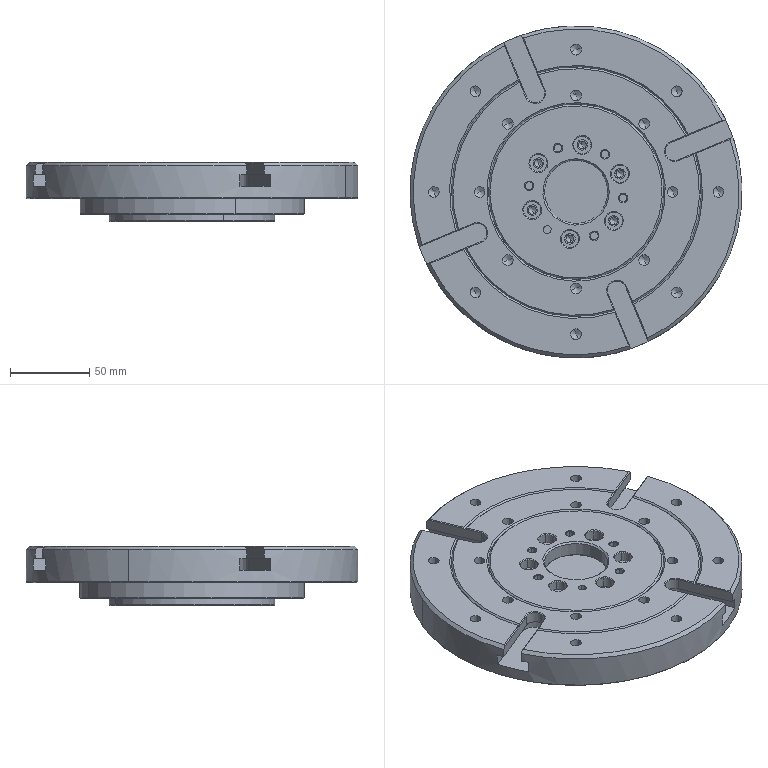NC program | Mastercam | posted with a generic post
Lines 3621 to 4738 of 4738:
(2.5 BM |TOOL - 15|DIA. OFF. - 15|LEN. - 15|TOOL DIA. - 2.5)
N7282 T15 M6
N7284 G0 G54 G90 X14.156 Y9.473 C49.947 B-90. S4500 M3
N7286 G43 H15 Z29.608
N7288 Y3.528
N7290 Z11.026
N7292 Z8.026
N7294 G1 Z6.026 F2000.
N7296 X14.166 Z5.862 F1000.
N7298 X14.193 Z5.699
N7300 X14.283 Z5.38
N7302 X14.292 Y3.524 Z5.322
N7304 X14.283 Y3.514 Z5.264
N7306 X14.22 Y3.48 Z5.155
N7308 X14.122 Y3.436 Z5.064
N7310 X14.012 Y3.391 Z5.007
N7312 X13.503 Y3.187 Z4.843 C50.063
N7314 X13.276 Y3.113 Z4.783 C50.113
N7316 X13.048 Y3.039 Z4.724 C50.163
N7318 X12.813 Y2.982 Z4.679 C50.213
N7320 X12.577 Y2.927 Z4.633 C50.234
N7322 X12.336 Y2.889 Z4.602 C50.255
N7324 X12.095 Y2.853 Z4.569 C50.247
N7326 X11.85 Y2.836 Z4.552 C50.24
N7328 X11.606 Y2.818 Z4.534 C50.232
N7330 X11.36 Z4.532 C50.224
N7332 X11.114 Y2.824 Z4.527 C50.161
N7334 X10.869 Y2.846 Z4.538 C50.098
N7336 X10.624 Y2.868 Z4.548 C50.035
N7338 X10.382 Y2.907 Z4.575 C49.971
N7340 X10.14 Y2.946 Z4.601 C49.908
N7342 X9.903 Y3. Z4.642 C49.845
N7344 X9.666 Y3.055 Z4.683 C49.782
N7346 X9.437 Y3.128 Z4.738 C49.719
N7348 X9.208 Y3.211 Z4.788 C49.558
N7350 X8.988 Y3.31 Z4.851 C49.398
N7352 X8.767 Y3.41 Z4.913 C49.237
N7354 X8.559 Y3.525 Z4.989 C49.077
N7356 X8.35 Y3.641 Z5.063 C48.916
N7358 X8.154 Y3.772 Z5.15 C48.755
N7360 X7.958 Y3.903 Z5.236 C48.595
N7362 X7.778 Y4.049 Z5.332 C48.434
N7364 X7.597 Y4.194 Z5.428 C48.274
N7366 X7.432 Y4.353 Z5.534 C48.113
N7368 X7.268 Y4.513 Z5.638 C47.953
N7370 X7.131 Y4.71 Z5.751 C47.785
N7372 X6.993 Y4.933 Z5.845 C47.412
N7374 X6.972 Y4.964 Z5.862 C47.357
N7376 X6.949 Y4.993 Z5.878 C47.301
N7378 X6.924 Y5.02 Z5.893 C47.246
N7380 X6.897 Y5.046 Z5.908 C47.191
N7382 X6.868 Y5.07 Z5.921 C47.136
N7384 X6.838 Y5.092 Z5.934 C47.081
N7386 X6.807 Y5.112 Z5.946 C47.026
N7388 X6.775 Y5.131 Z5.956 C46.971
N7390 X6.742 Y5.147 Z5.966 C46.917
N7392 X6.708 Y5.162 Z5.975 C46.863
N7394 X6.674 Y5.175 Z5.983 C46.81
N7396 X6.639 Y5.186 Z5.989 C46.756
N7398 X6.604 Y5.195 Z5.995 C46.703
N7400 X6.569 Y5.202 Z6. C46.651
N7402 X6.534 Y5.208 Z6.003 C46.599
N7404 X6.5 Y5.212 Z6.006 C46.547
N7406 X6.465 Y5.215 Z6.009 C46.496
N7408 X6.431 Y5.216 Z6.01 C46.445
N7410 X6.397 C46.394
N7412 X6.363 Y5.215 C46.344
N7414 X6.275 Y5.223 Z6.005 C46.216
N7416 X6.285 Y5.226 Z6.002 C46.202
N7418 X6.294 Y5.229 Z5.999 C46.189
N7420 X6.302 Y5.232 Z5.996 C46.176
N7422 X6.311 Y5.236 Z5.992 C46.162
N7424 X6.227 Y5.233 Z5.996 C46.035
N7426 X6.228 Y5.231 C46.03
N7428 X6.23 Y5.229 Z5.995 C46.026
N7430 X6.232 Y5.227 C46.022
N7432 X6.234 Y5.225 Z5.994 C46.017
N7434 X6.236 Y5.223 Z5.993 C46.013
N7436 X6.237 Y5.222 C46.009
N7438 X6.239 Y5.22 Z5.992 C46.004
N7440 X6.241 Y5.218 C46.
N7442 X6.243 Y5.216 Z5.991 C45.996
N7444 X6.244 Y5.214 Z5.99 C45.991
N7446 X6.246 Y5.212 C45.987
N7448 X6.248 Y5.21 Z5.989 C45.983
N7450 X6.25 Y5.209 C45.978
N7452 X6.251 Y5.207 Z5.988 C45.974
N7454 X6.253 Y5.205 C45.969
N7456 X6.255 Y5.203 Z5.987 C45.965
N7458 X6.257 Y5.201 Z5.986 C45.961
N7460 X6.259 Y5.199 C45.956
N7462 X6.26 Y5.197 Z5.985 C45.952
N7464 X6.262 Y5.196 C45.948
N7466 X6.264 Y5.194 Z5.984 C45.943
N7468 X6.266 Y5.192 Z5.983 C45.939
N7470 X6.267 Y5.19 C45.935
N7472 X6.269 Y5.188 Z5.982 C45.93
N7474 X6.271 Y5.186 C45.926
N7476 X6.273 Y5.184 Z5.981 C45.922
N7478 X6.274 Y5.183 C45.917
N7480 X6.276 Y5.181 Z5.98 C45.913
N7482 X6.278 Y5.179 Z5.979 C45.909
N7484 X6.28 Y5.177 C45.904
N7486 X6.281 Y5.175 Z5.978 C45.9
N7488 X6.283 Y5.169 Z5.976 C45.89
N7490 X6.284 Y5.164 Z5.974 C45.879
N7492 Y5.157 C45.867
N7494 Y5.151 C45.855
N7496 X6.287 Y5.15 Z5.97 C45.848
N7498 X6.29 Y5.149 Z5.966 C45.841
N7500 X6.293 Z5.961 C45.834
N7502 X6.296 Y5.148 Z5.957 C45.827
N7504 X6.299 Z5.953 C45.82
N7506 X6.307 Y5.152 Z5.957 C45.804
N7508 X6.276 Y5.097 Z5.989 C45.676
N7510 X6.278 Y5.096 Z5.986 C45.671
N7512 X6.281 Y5.095 Z5.984 C45.667
N7514 X6.283 Y5.094 Z5.982 C45.662
N7516 X6.285 Y5.093 Z5.98 C45.657
N7518 X6.287 Y5.092 Z5.978 C45.653
N7520 X6.289 Y5.09 Z5.976 C45.648
N7522 X6.297 Y5.077 Z5.972 C45.619
N7524 X6.305 Y5.063 Z5.969 C45.593
N7526 X6.298 Y4.73 Z6.205 C44.831
N7528 X6.303 Y4.403 Z6.404 C43.929
N7530 X6.309 Y4.055 Z6.603 C42.988
N7532 X6.321 Y3.757 Z6.758 C41.801
N7534 X6.341 Y3.441 Z6.91 C40.561
N7536 X6.373 Y3.158 Z7.033 C39.242
N7538 X6.415 Y2.862 Z7.153 C37.875
N7540 X6.47 Y2.596 Z7.255 C36.423
N7542 X6.555 Y2.322 Z7.333 C34.946
N7544 X6.652 Y2.101 Z7.396 C33.246
N7546 X6.768 Y1.878 Z7.455 C31.512
N7548 X6.913 Y1.686 Z7.493 C29.682
N7550 X7.079 Y1.501 Z7.527 C27.855
N7552 X7.266 Y1.325 Z7.557 C26.041
N7554 X7.325 Y1.282 Z7.562 C25.507
N7556 X7.344 Y1.273 Z7.563 C25.377
N7558 X7.363 Y1.265 Z7.562 C25.247
N7560 X7.383 Y1.258 Z7.558 C25.117
N7562 X7.403 Y1.251 Z7.551 C24.987
N7564 X7.424 Y1.247 Z7.541 C24.841
N7566 X7.444 Y1.244 Z7.529 C24.695
N7568 X7.465 Y1.242 Z7.515 C24.55
N7570 X7.485 Y1.241 Z7.499 C24.406
N7572 X7.505 Y1.24 Z7.482 C24.263
N7574 X7.525 Y1.241 Z7.462 C24.121
N7576 X7.545 Y1.243 Z7.442 C23.981
N7578 X7.564 Y1.246 Z7.42 C23.842
N7580 X7.582 Y1.251 Z7.398 C23.697
N7582 X7.601 Y1.257 Z7.374 C23.553
N7584 X7.618 Y1.264 Z7.35 C23.411
N7586 X7.635 Y1.272 Z7.326 C23.272
N7588 X7.81 Y1.274 Z7.077 C21.581
N7590 X7.975 Y1.291 Z6.846 C20.026
N7592 X8.12 Y1.293 Z6.662 C18.699
N7594 X8.28 Y1.286 Z6.465 C17.239
N7596 X8.447 Y1.251 Z6.276 C15.654
N7598 X8.6 Y1.196 Z6.092 C14.039
N7600 X8.672 Y1.149 Z6. C13.132
N7602 X8.745 Y1.106 Z5.912 C12.183
N7604 X8.852 Y1.012 Z5.763 C10.481
N7606 X8.937 Y.905 Z5.637 C8.736
N7608 X8.967 Y.836 Z5.584 C7.762
N7610 X8.997 Y.766 Z5.535 C6.787
N7612 X9.026 Y.634 Z5.465 C5.054
N7614 X9.025 Y.557 Z5.444 C4.088
N7616 X9.024 Y.481 Z5.427 C3.104
N7618 X8.993 Y.349 Z5.424 C1.364
N7620 X8.961 Y.276 Z5.435 C.415
N7622 X8.929 Y.202 Z5.45 C-.522
N7624 X8.843 Y.082 Z5.504 C-2.172
N7626 X8.737 Y-.024 Z5.576 C-3.805
N7628 X8.664 Y-.074 Z5.628 C-4.715
N7630 X8.59 Y-.122 Z5.684 C-5.626
N7632 X8.437 Y-.181 Z5.804 C-7.217
N7634 X8.188 Y-.254 Z6.015 C-9.499
N7636 X8.006 Y-.311 Z6.18 C-11.258
N7638 X7.923 Y-.333 Z6.264 C-12.084
N7640 X7.754 Y-.385 Z6.44 C-13.835
N7642 X7.669 Y-.419 Z6.536 C-14.696
N7644 X7.515 Y-.482 Z6.721 C-16.317
N7646 X7.373 Y-.543 Z6.912 C-17.934
N7648 X7.221 Y-.608 Z7.138 C-19.793
N7650 X7.157 Y-.599 Z7.2 C-20.143
N7652 X7.093 Y-.59 Z7.263 C-20.492
N7654 X7.028 Y-.579 Z7.326 C-20.841
N7656 X6.964 Y-.568 Z7.389 C-21.191
N7658 X6.899 Y-.556 Z7.452 C-21.54
N7660 X6.799 Y-.66 Z7.578 C-22.685
N7662 X6.793 Y-.674 Z7.593 C-22.82
N7664 X6.788 Y-.689 Z7.605 C-22.956
N7666 X6.783 Y-.704 Z7.614 C-23.091
N7668 X6.779 Y-.72 Z7.62 C-23.226
N7670 X6.775 Y-.737 Z7.624 C-23.361
N7672 X6.772 Y-.753 C-23.495
N7674 X6.77 Y-.769 Z7.622 C-23.629
N7676 X6.769 Y-.785 Z7.618 C-23.761
N7678 X6.768 Y-.8 Z7.612 C-23.893
N7680 Y-.815 Z7.604 C-24.023
N7682 X6.69 Y-.963 Z7.591 C-25.313
N7684 X6.621 Y-1.175 Z7.565 C-26.337
N7686 X6.564 Y-1.388 Z7.529 C-27.363
N7688 X6.516 Y-1.628 Z7.48 C-28.317
N7690 X6.47 Y-1.871 Z7.431 C-29.101
N7692 X6.437 Y-2.122 Z7.364 C-29.918
N7694 X6.403 Y-2.384 Z7.293 C-30.608
N7696 X6.376 Y-2.661 Z7.209 C-31.188
N7698 X6.352 Y-2.936 Z7.118 C-31.766
N7700 X6.341 Y-3.256 Z6.985 C-32.085
N7702 X6.327 Y-3.566 Z6.852 C-32.396
N7704 X6.32 Y-3.869 Z6.705 C-32.707
N7706 X6.31 Y-4.169 Z6.551 C-33.017
N7708 X6.304 Y-4.484 Z6.372 C-33.191
N7710 X6.295 Y-4.598 Z6.319 C-33.251
N7712 X6.293 Y-4.604 C-33.255
N7714 X6.291 Y-4.611 Z6.32 C-33.258
N7716 X6.289 Y-4.618 C-33.261
N7718 X6.287 Y-4.624 C-33.264
N7720 X6.285 Y-4.631 C-33.268
N7722 X6.283 Y-4.637 C-33.271
N7724 X6.281 Y-4.644 C-33.274
N7726 X6.279 Y-4.651 Z6.321 C-33.278
N7728 X6.277 Y-4.657 C-33.281
N7730 X6.275 Y-4.664 C-33.284
N7732 X6.273 Y-4.67 C-33.287
N7734 X6.271 Y-4.677 C-33.291
N7736 X6.269 Y-4.684 C-33.294
N7738 X6.267 Y-4.69 Z6.322 C-33.297
N7740 X6.266 Y-4.697 C-33.3
N7742 X6.264 Y-4.703 C-33.304
N7744 X6.262 Y-4.71 C-33.307
N7746 X6.26 Y-4.716 C-33.31
N7748 X6.258 Y-4.723 C-33.313
N7750 X6.256 Y-4.73 Z6.323 C-33.317
N7752 X6.254 Y-4.736 C-33.32
N7754 X6.252 Y-4.743 C-33.323
N7756 X6.312 Y-4.767 Z6.305 C-33.354
N7758 X6.319 Y-4.77 C-33.358
N7760 X6.325 Y-4.774 C-33.361
N7762 X7.175 Y-5.239 Z6.286 C-33.808
N7764 X7.319 Y-5.324 Z6.287
N7766 X7.474 Y-5.413 Z6.309
N7768 X7.63 Y-5.5 Z6.352
N7770 X7.782 Y-5.58 Z6.416
N7772 X7.922 Y-5.65 Z6.5
N7774 X8.042 Y-5.706 Z6.605
N7776 X8.135 Y-5.742 Z6.73
N7778 X8.194 Y-5.756 Z6.875
N7780 X8.291 Z7.279
N7782 X8.37 Z7.687
N7784 X8.423 Z8.098
N7786 X8.443 Z8.511
N7788 G0 Z10.511
N7790 Z13.511
N7792 Z28.6
N7794 Y-12.184
N7796 Z30.435
N7798 X7.794 Y6.335
N7800 C-78.812
N7802 Y3.076
N7804 Z14.777
N7806 Z11.777
N7808 G1 Z9.777 F2000.
N7810 X7.766 Z9.367 F1000.
N7812 X7.691 Z8.962
N7814 X7.579 Z8.563
N7816 X7.444 Z8.173
N7818 X7.384 Y3.051 Z8.043
N7820 X7.311 Y2.984 Z7.932
N7822 X7.229 Y2.883 Z7.841
N7824 X7.143 Y2.755 Z7.77
N7826 X7.057 Y2.611 Z7.719
N7828 X6.974 Y2.458 Z7.689
N7830 X6.898 Y2.304 Z7.679
N7832 X6.834 Y2.16 Z7.69
N7834 X6.789 Y2.083 Z7.698 C-79.057
N7836 X6.744 Y2.01 Z7.705 C-79.331
N7838 X6.699 Y1.938 Z7.714 C-79.606
N7840 X6.654 Y1.866 Z7.724 C-79.88
N7842 X6.609 Y1.798 Z7.734 C-80.18
N7844 X6.563 Y1.73 Z7.744 C-80.481
N7846 X6.518 Y1.669 Z7.755 C-80.817
N7848 X6.473 Y1.607 Z7.766 C-81.154
N7850 X6.442 Y1.565 Z7.775 C-81.384
N7852 X6.412 Y1.523 Z7.784 C-81.613
N7854 X6.381 Y1.452 Z7.791 C-81.979
N7856 X6.343 Y1.395 Z7.802 C-82.297
N7858 X6.305 Y1.337 Z7.813 C-82.614
N7860 X6.276 Y1.266 Z7.82 C-83.021
N7862 X6.243 Y1.209 Z7.829 C-83.356
N7864 X6.21 Y1.157 Z7.839 C-83.721
N7866 X6.187 Y1.09 Z7.843 C-84.157
N7868 X6.16 Y1.038 Z7.851 C-84.513
N7870 X6.133 Y.972 Z7.859 C-84.951
N7872 X6.111 Y.917 Z7.864 C-85.301
N7874 X6.089 Y.863 Z7.871 C-85.652
N7876 X6.067 Y.809 Z7.878 C-86.003
N7878 X6.052 Y.743 Z7.881 C-86.446
N7880 X6.035 Y.69 Z7.886 C-86.801
N7882 X6.018 Y.641 Z7.892 C-87.178
N7884 X6.004 Y.578 Z7.895 C-87.651
N7886 X5.992 Y.528 Z7.898 C-88.029
N7888 X5.981 Y.465 Z7.902 C-88.504
N7890 X5.974 Y.413 Z7.904 C-88.867
N7892 X5.967 Y.361 Z7.906 C-89.23
N7894 X5.959 Y.309 Z7.91 C-89.593
N7896 X5.955 Y.244 Z7.911 C-90.055
N7898 X5.952 Y.192 Z7.913 C-90.421
N7900 X5.95 Y.141 Z7.915 C-90.788
N7902 X5.954 Y.076 Z7.914 C-91.255
N7904 X5.957 Y.024 C-91.624
N7906 X5.96 Y-.04 Z7.915 C-92.09
N7908 X5.967 Y-.088 Z7.913 C-92.479
N7910 X5.974 Y-.136 Z7.912 C-92.868
N7912 X5.981 Y-.183 C-93.257
N7914 X5.994 Y-.244 Z7.909 C-93.742
N7916 X6.006 Y-.293 Z7.907 C-94.129
N7918 X6.018 Y-.341 C-94.516
N7920 X6.035 Y-.401 Z7.903 C-95.003
N7922 X6.052 Y-.449 Z7.9 C-95.393
N7924 X6.069 Y-.497 Z7.898 C-95.783
N7926 X6.091 Y-.558 Z7.894 C-96.265
N7928 X6.113 Y-.606 Z7.889 C-96.654
N7930 X6.135 Y-.655 Z7.886 C-97.043
N7932 X6.16 Y-.715 Z7.882 C-97.52
N7934 X6.187 Y-.765 Z7.876 C-97.89
N7936 X6.214 Y-.815 Z7.872 C-98.26
N7938 X6.244 Y-.878 Z7.867 C-98.722
N7940 X6.277 Y-.928 Z7.86 C-99.105
N7942 X6.31 Y-.978 Z7.855 C-99.487
N7944 X6.343 Y-1.039 Z7.849 C-99.948
N7946 X6.381 Y-1.09 Z7.841 C-100.313
N7948 X6.419 Y-1.14 Z7.835 C-100.678
N7950 X6.447 Y-1.208 Z7.833 C-101.116
N7952 X6.486 Y-1.25 Z7.825 C-101.432
N7954 X6.525 Y-1.293 Z7.817 C-101.748
N7956 X6.563 Y-1.335 Z7.81 C-102.064
N7958 X6.603 Y-1.388 Z7.803 C-102.436
N7960 X6.646 Y-1.43 Z7.795 C-102.748
N7962 X6.689 Y-1.471 Z7.787 C-103.06
N7964 X6.726 Y-1.525 Z7.781 C-103.391
N7966 X6.77 Y-1.564 Z7.772 C-103.668
N7968 X6.814 Y-1.605 Z7.763 C-103.929
N7970 X6.859 Y-1.647 Z7.754 C-104.191
N7972 X6.899 Y-1.703 Z7.748 C-104.518
N7974 X6.949 Y-1.741 Z7.738 C-104.794
N7976 X6.999 Y-1.78 Z7.729 C-105.07
N7978 X7.036 Y-1.838 Z7.726 C-105.398
N7980 X7.091 Y-1.878 Z7.714 C-105.654
N7982 X7.147 Y-1.919 Z7.703 C-105.91
N7984 X7.203 Y-1.96 Z7.692 C-106.164
N7986 X7.258 Y-2. Z7.681 C-106.418
N7988 X7.309 Y-2.055 Z7.673 C-106.706
N7990 X7.369 Y-2.092 Z7.662 C-106.961
N7992 X7.429 Y-2.13 Z7.65 C-107.21
N7994 X7.479 Y-2.185 Z7.644 C-107.484
N7996 X7.542 Y-2.219 Z7.632 C-107.73
N7998 X7.606 Y-2.254 Z7.62 C-107.976
N8000 X7.657 Y-2.308 Z7.612 C-108.216
N8002 X7.724 Y-2.344 Z7.6 C-108.441
N8004 X7.79 Y-2.38 Z7.587 C-108.666
N8006 X7.857 Y-2.415 Z7.575 C-108.892
N8008 X7.917 Y-2.461 Z7.566 C-109.125
N8010 X7.986 Y-2.493 Z7.554 C-109.35
N8012 X8.043 Y-2.541 Z7.546 C-109.582
N8014 X8.112 Y-2.569 Z7.534 C-109.793
N8016 X8.18 Y-2.597 Z7.523 C-110.005
N8018 X8.249 Y-2.628 Z7.512 C-110.202
N8020 X8.299 Y-2.679 Z7.506 C-110.409
N8022 X8.38 Y-2.71 Z7.493 C-110.633
N8024 X8.461 Y-2.741 Z7.48 C-110.857
N8026 X8.542 Y-2.774 Z7.467 C-111.066
N8028 X8.616 Y-2.815 Z7.456 C-111.271
N8030 X8.7 Y-2.845 Z7.443 C-111.479
N8032 X8.784 Y-2.876 Z7.43 C-111.683
N8034 X8.845 Y-2.908 Z7.422 C-111.844
N8036 X8.915 Y-2.931 Z7.412 C-112.009
N8038 X8.986 Y-2.954 Z7.402 C-112.173
N8040 X9.057 Y-2.998 Z7.394 C-112.37
N8042 X9.147 Y-3.023 Z7.382 C-112.573
N8044 X9.237 Y-3.048 Z7.37 C-112.776
N8046 X9.311 Y-3.085 Z7.362 C-112.963
N8048 X9.404 Y-3.105 Z7.351 C-113.165
N8050 X9.496 Y-3.13 Z7.339 C-113.33
N8052 X9.589 Y-3.156 Z7.327 C-113.495
N8054 X9.666 Y-3.197 Z7.317 C-113.653
N8056 X9.76 Y-3.226 Z7.306 C-113.822
N8058 X9.865 Y-3.252 Z7.293 C-113.979
N8060 X9.969 Y-3.277 Z7.28 C-114.136
N8062 X10.055 Y-3.316 Z7.27 C-114.279
N8064 X10.167 Y-3.338 Z7.258 C-114.443
N8066 X10.278 Y-3.36 Z7.246 C-114.607
N8068 X10.37 Y-3.394 Z7.237 C-114.752
N8070 X10.465 Y-3.409 Z7.228 C-114.89
N8072 X10.559 Y-3.424 Z7.219 C-115.027
N8074 X10.654 Y-3.439 Z7.211 C-115.164
N8076 X10.728 Y-3.466 Z7.205 C-115.28
N8078 X10.825 Y-3.477 Z7.198 C-115.418
N8080 X10.921 Y-3.489 Z7.191 C-115.556
N8082 X11.018 Y-3.5 Z7.184 C-115.694
N8084 X11.098 Y-3.526 Z7.179 C-115.817
N8086 X11.211 Y-3.536 Z7.173 C-115.976
N8088 X11.313 Y-3.547 Z7.168 C-116.12
N8090 X11.426 Y-3.556 Z7.161 C-116.263
N8092 X11.522 Y-3.574 Z7.156 C-116.388
N8094 X11.63 Y-3.585 Z7.15 C-116.492
N8096 X11.739 Y-3.595 Z7.144 C-116.597
N8098 X11.828 Y-3.614 Z7.138 C-116.667
N8100 X11.926 Y-3.623 Z7.132 C-116.742
N8102 X12.025 Y-3.632 Z7.127 C-116.812
N8104 X12.123 Y-3.642 Z7.121 C-116.882
N8106 X12.199 Y-3.657 Z7.117 C-116.937
N8108 X12.298 Y-3.663 Z7.113 C-117.007
N8110 X12.397 Y-3.669 Z7.11 C-117.077
N8112 X12.496 Y-3.674 Z7.106 C-117.147
N8114 X12.595 Y-3.68 Z7.102 C-117.216
N8116 X12.672 Y-3.688 Z7.101 C-117.271
N8118 X12.771 Y-3.69 Z7.099 C-117.34
N8120 X12.87 Y-3.692 Z7.097 C-117.41
N8122 X12.947 Y-3.703 Z7.096 C-117.464
N8124 X13.047 Y-3.702 C-117.534
N8126 X13.146 Y-3.701 Z7.095 C-117.603
N8128 X13.246 Y-3.699 C-117.673
N8130 X13.323 Y-3.708 C-117.728
N8132 X13.423 Y-3.703 Z7.097 C-117.797
N8134 X13.522 Y-3.698 Z7.099 C-117.866
N8136 X13.622 Y-3.694 Z7.1 C-117.935
N8138 X13.699 Y-3.695 Z7.102 C-117.989
N8140 X13.799 Y-3.687 Z7.105 C-118.059
N8142 X13.9 Y-3.678 Z7.109 C-118.128
N8144 X14. Y-3.67 Z7.112 C-118.198
N8146 X14.1 Y-3.661 Z7.116 C-118.267
N8148 X14.213 Y-3.652 Z7.121 C-118.346
N8150 X14.338 Y-3.641 Z7.126 C-118.421
N8152 X14.462 Y-3.63 Z7.13 C-118.497
N8154 X14.586 Y-3.623 Z7.133 C-118.54
N8156 X14.711 Y-3.617 Z7.136 C-118.583
N8158 X14.835 Y-3.615 Z7.137 C-118.594
N8160 X14.959 Y-3.614 C-118.604
N8162 X15.084
N8164 X15.208
N8166 X15.332
N8168 X15.457
N8170 X15.581
N8172 X15.705
N8174 X15.83
N8176 X15.954
N8178 X16.078
N8180 X16.203
N8182 X16.327
N8184 X16.451
N8186 X15.879 Y-3.699 Z7.207 C-118.726
N8188 X16.004 Y-3.694 Z7.209 C-118.768
N8190 X16.129 Y-3.688 Z7.211 C-118.811
N8192 X16.254 Y-3.683 Z7.214 C-118.853
N8194 X16.379 Y-3.672 Z7.218 C-118.932
N8196 X16.504 Y-3.661 Z7.223 C-119.012
N8198 X16.629 Y-3.65 Z7.227 C-119.091
N8200 X16.754 Y-3.633 Z7.234 C-119.208
N8202 X16.879 Y-3.616 Z7.241 C-119.325
N8204 X17.004 Y-3.6 Z7.248 C-119.442
N8206 X17.109 Y-3.583 Z7.255 C-119.573
N8208 X17.253 Y-3.56 Z7.263 C-119.754
N8210 X17.367 Y-3.549 Z7.267 C-119.897
N8212 X17.521 Y-3.523 Z7.275 C-120.155
N8214 X17.635 Y-3.512 Z7.278 C-120.348
N8216 X17.789 Y-3.495 Z7.282 C-120.609
N8218 X17.902 Y-3.476 Z7.288 C-120.904
N8220 X18.055 Y-3.447 Z7.295 C-121.304
N8222 X18.166 Y-3.434 Z7.298 C-121.6
N8224 X18.318 Y-3.403 Z7.306 C-122.08
N8226 X18.427 Y-3.389 Z7.309 C-122.434
N8228 X18.536 Y-3.374 Z7.312 C-122.787
N8230 X18.684 Y-3.348 Z7.317 C-123.358
N8232 X18.831 Y-3.325 Z7.322 C-123.932
N8234 X18.935 Y-3.313 C-124.349
N8236 X19.039 Y-3.292 Z7.327 C-124.827
N8238 X19.174 Y-3.262 Z7.329 C-125.448
N8240 X19.305 Y-3.247 Z7.332 C-126.083
N8242 X19.376 Y-3.23 Z7.335 C-126.489
N8244 X19.447 Y-3.214 Z7.338 C-126.896
N8246 X19.56 Y-3.187 Z7.341 C-127.541
N8248 X19.655 Y-3.169 Z7.343 C-128.108
N8250 X19.79 Y-3.136 Z7.347 C-128.963
N8252 X19.881 Y-3.118 Z7.349 C-129.563
N8254 X19.972 Y-3.1 Z7.35 C-130.163
N8256 X20.088 Y-3.072 Z7.352 C-130.997
N8258 X20.166 Y-3.055 Z7.354 C-131.572
N8260 X20.263 Y-3.038 C-132.323
N8262 X20.324 Y-3.025 Z7.355 C-132.804
N8264 X20.384 Y-3.013 Z7.356 C-133.285
N8266 X20.502 Y-2.99 Z7.354 C-134.253
N8268 X20.579 Y-2.974 Z7.355 C-134.929
N8270 X20.675 Y-2.956 Z7.353 C-135.804
N8272 X20.731 Y-2.946 Z7.352 C-136.33
N8274 X20.786 Y-2.938 C-136.856
N8276 X20.885 Y-2.92 Z7.349 C-137.842
N8278 X20.947 Y-2.911 Z7.348 C-138.474
N8280 X21.036 Y-2.898 Z7.343 C-139.428
N8282 X21.093 Y-2.891 Z7.341 C-140.058
N8284 X21.167 Y-2.883 Z7.334 C-140.903
N8286 X21.207 Y-2.879 Z7.332 C-141.39
N8288 X21.246 Y-2.876 Z7.33 C-141.878
N8290 X21.268 Y-2.873 Z7.326 C-142.152
N8292 X21.296 Y-2.253 Z7.512 C-146.739
N8294 X21.324 Y-1.621 Z7.645 C-151.327
N8296 X21.351 Y-.983 Z7.726 C-155.914
N8298 X21.379 Y-.342 Z7.753 C-160.502
N8300 X21.388 Y-.344 Z7.749 C-160.797
N8302 X21.392 Y-.351 Z7.745 C-161.525
N8304 X21.395 Y-.36 Z7.742 C-162.241
N8306 X21.399 Y-.369 C-162.957
N8308 X21.403 Y-.38 C-163.661
N8310 X21.406 Y-.391 Z7.745 C-164.365
N8312 X21.411 Y-.419 Z7.741 C-165.36
N8314 X21.415 Y-.436 Z7.738 C-166.015
N8316 X21.419 Y-.453 Z7.737 C-166.67
N8318 X21.423 Y-.47 C-167.331
N8320 X21.428 Y-.495 Z7.74 C-168.344
N8322 X21.433 Y-.511 Z7.735 C-169.01
N8324 X21.437 Y-.527 Z7.732 C-169.675
N8326 X21.441 Y-.542 Z7.731 C-170.341
N8328 X21.446 Y-.561 C-170.989
N8330 X21.45 Y-.579 Z7.732 C-171.637
N8332 X21.456 Y-.608 Z7.728 C-172.631
N8334 X21.461 Y-.63 Z7.724 C-173.256
N8336 X21.466 Y-.652 Z7.722 C-173.881
N8338 X21.471 Y-.674 C-174.506
N8340 X21.476 Y-.704 Z7.723 C-175.35
N8342 X21.481 Y-.724 Z7.721 C-175.928
N8344 X21.485 Y-.749 Z7.719 C-176.481
N8346 X21.49 Y-.773 C-177.034
N8348 X21.495 Y-.798 Z7.72 C-177.586
N8350 X21.499 Y-.822 Z7.722 C-178.139
N8352 X21.504 Y-.847 Z7.726 C-178.692
N8354 X21.509 Y-.885 Z7.734 C-179.534
N8356 X21.514 Y-.909 Z7.733 C-180.087
N8358 X21.519 Y-.936 Z7.734 C-180.622
N8360 X21.524 Y-.963 Z7.736 C-181.158
N8362 X21.529 Y-.99 Z7.739 C-181.693
N8364 X21.534 Y-1.017 Z7.743 C-182.228
N8366 X21.539 Y-1.045 Z7.749 C-182.764
N8368 X21.546 Y-1.086 Z7.759 C-183.579
N8370 X21.551 Y-1.113 Z7.761 C-184.115
N8372 X21.556 Y-1.142 Z7.763 C-184.633
N8374 X21.561 Y-1.172 Z7.767 C-185.152
N8376 X21.567 Y-1.204 Z7.772 C-185.654
N8378 X21.572 Y-1.236 Z7.777 C-186.156
N8380 X21.577 Y-1.268 Z7.785 C-186.658
N8382 X21.583 Y-1.317 Z7.798 C-187.423
N8384 X21.588 Y-1.349 Z7.801 C-187.924
N8386 X21.594 Y-1.38 Z7.805 C-188.426
N8388 X21.599 Y-1.412 Z7.81 C-188.928
N8390 X21.604 Y-1.444 Z7.817 C-189.429
N8392 X21.61 Y-1.476 Z7.825 C-189.931
N8394 X21.615 Y-1.507 Z7.834 C-190.433
N8396 X21.621 Y-1.539 Z7.844 C-190.934
N8398 X21.629 Y-1.587 Z7.853 C-191.699
N8400 X21.634 Y-1.618 Z7.859 C-192.201
N8402 X21.64 Y-1.65 Z7.867 C-192.702
N8404 X21.646 Y-1.681 Z7.875 C-193.204
N8406 X21.651 Y-1.712 Z7.885 C-193.705
N8408 X21.657 Y-1.743 Z7.896 C-194.207
N8410 X21.663 Y-1.774 Z7.908 C-194.708
N8412 X21.671 Y-1.821 Z7.921 C-195.473
N8414 X21.677 Y-1.852 Z7.929 C-195.975
N8416 X21.683 Y-1.883 Z7.938 C-196.476
N8418 X21.688 Y-1.913 Z7.948 C-196.978
N8420 X21.694 Y-1.944 Z7.96 C-197.48
N8422 X21.7 Y-1.974 Z7.973 C-197.983
N8424 X21.706 Y-2.005 Z7.987 C-198.485
N8426 X21.712 Y-2.051 Z8.004 C-199.251
N8428 X21.718 Y-2.08 Z8.014 C-199.754
N8430 X21.724 Y-2.11 Z8.025 C-200.256
N8432 X21.73 Y-2.14 Z8.038 C-200.758
N8434 X21.736 Y-2.17 Z8.051 C-201.261
N8436 X21.742 Y-2.199 Z8.066 C-201.763
N8438 X21.748 Y-2.228 Z8.082 C-202.267
N8440 X21.756 Y-2.273 Z8.1 C-203.036
N8442 X21.763 Y-2.301 Z8.112 C-203.54
N8444 X21.769 Y-2.33 Z8.125 C-204.043
N8446 X21.775 Y-2.359 Z8.139 C-204.547
N8448 X21.781 Y-2.387 Z8.154 C-205.051
N8450 X21.787 Y-2.416 Z8.171 C-205.555
N8452 X21.793 Y-2.444 Z8.189 C-206.058
N8454 X21.801 Y-2.487 Z8.21 C-206.828
N8456 X21.808 Y-2.514 Z8.224 C-207.333
N8458 X21.814 Y-2.542 Z8.238 C-207.838
N8460 X21.82 Y-2.569 Z8.254 C-208.343
N8462 X21.826 Y-2.596 Z8.272 C-208.848
N8464 X21.833 Y-2.624 Z8.29 C-209.354
N8466 X21.839 Y-2.651 Z8.31 C-209.859
N8468 X21.846 Y-2.692 Z8.335 C-210.631
N8470 X21.852 Y-2.718 Z8.35 C-211.136
N8472 X21.858 Y-2.744 Z8.367 C-211.641
N8474 X21.865 Y-2.77 Z8.385 C-212.152
N8476 X21.871 Y-2.795 Z8.404 C-212.662
N8478 X21.877 Y-2.82 Z8.424 C-213.173
N8480 X21.884 Y-2.845 Z8.446 C-213.684
N8482 X21.892 Y-2.882 Z8.472 C-214.465
N8484 X21.899 Y-2.907 Z8.49 C-214.975
N8486 X21.905 Y-2.931 Z8.508 C-215.486
N8488 X21.912 Y-2.955 Z8.527 C-215.997
N8490 X21.918 Y-2.979 Z8.548 C-216.507
N8492 X21.924 Y-3. Z8.571 C-217.033
N8494 X21.931 Y-3.021 Z8.595 C-217.56
N8496 X21.939 Y-3.052 Z8.626 C-218.365
N8498 X21.946 Y-3.072 Z8.645 C-218.891
N8500 X21.952 Y-3.092 Z8.666 C-219.417
N8502 X21.959 Y-3.112 Z8.688 C-219.944
N8504 X21.965 Y-3.132 Z8.711 C-220.47
N8506 X21.971 Y-3.155 Z8.734 C-220.979
N8508 X21.978 Y-3.177 Z8.759 C-221.488
N8510 X21.987 Y-3.211 Z8.79 C-222.267
N8512 X21.993 Y-3.236 Z8.809 C-222.753
N8514 X21.999 Y-3.262 Z8.829 C-223.239
N8516 X22.006 Y-3.287 Z8.85 C-223.726
N8518 X22.012 Y-3.313 Z8.873 C-224.212
N8520 X22.019 Y-3.338 Z8.896 C-224.698
N8522 X22.025 Y-3.363 Z8.921 C-225.184
N8524 X22.034 Y-3.401 Z8.952 C-225.929
N8526 X22.041 Y-3.431 Z8.97 C-226.383
N8528 X22.047 Y-3.461 Z8.989 C-226.837
N8530 X22.053 Y-3.496 Z9.008 C-227.259
N8532 X22.06 Y-3.532 Z9.027 C-227.68
N8534 X22.066 Y-3.567 Z9.048 C-228.102
N8536 X22.072 Y-3.603 Z9.069 C-228.523
N8538 X22.066 Y-3.633 Z9.096 C-228.887
N8540 X22.06 Y-3.663 Z9.124 C-229.25
N8542 X22.052 Y-3.702 Z9.161 C-229.723
N8544 X22.044 Y-3.74 Z9.2 C-230.196
N8546 X22.036 Y-3.778 Z9.24 C-230.668
N8548 X22.028 Y-3.816 Z9.281 C-231.141
N8550 X22.02 Y-3.853 Z9.324 C-231.614
N8552 X22.012 Y-3.89 Z9.368 C-232.086
N8554 X22.004 Y-3.926 Z9.413 C-232.559
N8556 X21.996 Y-3.962 Z9.46 C-233.032
N8558 X21.993 Y-4.121 Z9.489
N8560 X22.006 Y-4.287 Z9.535
N8562 X22.034 Y-4.453 Z9.597
N8564 X22.076 Y-4.608 Z9.672
N8566 X22.133 Y-4.745 Z9.758
N8568 X22.205 Y-4.854 Z9.854
N8570 X22.291 Y-4.926 Z9.957
N8572 X22.391 Y-4.952 Z10.065
N8574 X22.651 Z10.365
N8576 X22.769 Z10.53
N8578 X22.873 Z10.703
N8580 X22.961 Z10.883
N8582 X23.028 Z11.068
N8584 X23.071 Z11.257
N8586 X23.087 Z11.45
N8588 G0 Z13.45
N8590 Z16.45
N8592 Z29.768
N8594 Y-8.96
N8596 Z31.036
N8598 X-17.141 Y-8.869
N8600 C-180. B-270.
N8602 Z6.928
N8604 Z3.928
N8606 G1 Z1.928 F2000.
N8608 X-17.127 Y-8.867 Z1.734 F1000.
N8610 X-17.086 Y-8.862 Z1.542
N8612 X-17.023 Y-8.854 Z1.355
N8614 X-16.939 Y-8.844 Z1.172
N8616 X-16.84 Y-8.831 Z.996
N8618 X-16.728 Y-8.817 Z.827
N8620 X-16.479 Y-8.785 Z.517
N8622 X-16.383 Y-8.747 Z.413
N8624 X-16.295 Y-8.664 Z.327
N8626 X-16.215 Y-8.544 Z.259
N8628 X-16.147 Y-8.399 Z.206
N8630 X-16.089 Y-8.236 Z.171
N8632 X-16.046 Y-8.066 Z.152
N8634 X-16.016 Y-7.897 Z.149
N8636 X-16.003 Y-7.74 Z.163
N8638 X-15.985 Y-7.246 Z.234
N8640 X-15.968 Y-6.751 Z.305
N8642 X-15.95 Y-6.258 Z.376
N8644 X-15.933 Y-5.765 Z.447
N8646 X-15.916 Y-5.273 Z.518
N8648 X-15.898 Y-4.78 Z.589
N8650 X-15.897 Y-4.742 Z.594
N8652 X-15.896 Y-4.704 Z.597
N8654 X-15.895 Y-4.665 Z.598
N8656 X-15.894 Y-4.627 Z.597
N8658 X-15.893 Y-4.589 Z.594
N8660 Y-4.551 Z.59
N8662 Y-4.513 Z.583
N8664 X-15.894 Y-4.476 Z.575
N8666 Y-4.438 Z.565
N8668 X-15.895 Y-4.402 Z.554
N8670 X-15.896 Y-4.366 Z.541
N8672 X-15.897 Y-4.33 Z.526
N8674 X-15.899 Y-4.296 Z.509
N8676 X-15.905 Y-4.19 Z.453
N8678 X-15.91 Y-4.075 Z.401
N8680 X-15.915 Y-3.955 Z.356
N8682 X-15.916 Y-3.911 Z.342
N8684 X-15.918 Y-3.867 Z.327
N8686 X-15.919 Y-3.741 Z.297
N8688 X-15.92 Y-3.612 Z.274
N8690 Y-3.565 Z.268
N8692 Y-3.518 Z.262
N8694 X-15.918 Y-3.388 Z.255
N8696 X-15.916 Y-3.257 Z.256
N8698 X-15.914 Y-3.21 Z.259
N8700 X-15.912 Y-3.163 Z.263
N8702 X-15.907 Y-3.035 Z.28
N8704 X-15.901 Y-2.91 Z.304
N8706 X-15.898 Y-2.873 Z.314
N8708 X-15.895 Y-2.836 Z.323
N8710 X-15.887 Y-2.683 Z.372
N8712 X-15.884 Y-2.64 Z.386
N8714 X-15.881 Y-2.605 Z.388
N8716 Y-2.572 Z.393
N8718 Y-2.537 Z.398
N8720 X-15.88 Y-2.502 Z.402
N8722 X-15.879 Y-2.465 Z.405
N8724 X-15.877 Y-2.428 Z.408
N8726 X-15.874 Y-2.389 Z.41
N8728 X-15.871 Y-2.349 Z.411
N8730 X-15.867 Y-2.307
N8732 X-15.821 Y-2.228 Z.442
N8734 X-15.785 Y-2.19 Z.468
N8736 X-15.74 Y-2.113 Z.503
N8738 X-15.704 Y-2.073 Z.533
N8740 X-15.669 Y-2.034 Z.562
N8742 X-15.625 Y-1.96 Z.604
N8744 X-15.59 Y-1.924 Z.638
N8746 X-15.557 Y-1.889 Z.671
N8748 X-15.515 Y-1.819 Z.719
N8750 X-15.483 Y-1.787 Z.755
N8752 X-15.452 Y-1.756 Z.79
N8754 X-15.424 Y-1.737 Z.819
N8756 X-15.386 Y-1.675 Z.877
N8758 X-15.337 Y-1.596 Z.951
N8760 X-15.327 Y-1.558 Z.98
N8762 X-15.317 Y-1.517 Z1.004
N8764 X-15.307 Y-1.474 Z1.025
N8766 X-15.295 Y-1.43 Z1.042
N8768 X-15.284 Y-1.385 Z1.056
N8770 X-15.272 Y-1.339 Z1.065
N8772 X-15.26 Y-1.292 Z1.071
N8774 X-15.249 Y-1.246 Z1.073
N8776 X-15.238 Y-1.2
N8778 X-15.227 Y-1.154 Z1.069
N8780 X-15.217 Y-1.109 Z1.063
N8782 X-15.088 Y-.879 Z1.096
N8784 X-14.959 Y-.648 Z1.13
N8786 X-14.911 Y-.545 Z1.145
N8788 X-14.904 Y-.514 Z1.149
N8790 X-14.897 Y-.484 Z1.153
N8792 X-14.893 Y-.454 Z1.158
N8794 X-14.89 Y-.423 Z1.162
N8796 Y-.392 Z1.167
N8798 Y-.361 Z1.171
N8800 X-14.894 Y-.331 Z1.175
N8802 X-14.897 Y-.3 Z1.18
N8804 X-14.905 Y-.27 Z1.184
N8806 X-14.912 Y-.24 Z1.188
N8808 X-14.922 Y-.212 Z1.193
N8810 X-14.933 Y-.183 Z1.197
N8812 X-14.946 Y-.155 Z1.201
N8814 X-14.96 Y-.128 Z1.205
N8816 X-14.977 Y-.102 Z1.208
N8818 X-14.993 Y-.076 Z1.212
N8820 X-15.013 Y-.053 Z1.216
N8822 X-15.032 Y-.029 Z1.219
N8824 X-15.054 Y-.007 Z1.222
N8826 X-15.077 Y.014 Z1.225
N8828 X-15.101 Y.033 Z1.228
N8830 X-15.125 Y.051 Z1.231
N8832 X-15.152 Y.067 Z1.233
N8834 X-15.178 Y.083 Z1.235
N8836 X-15.206 Y.096 Z1.237
N8838 X-15.234 Y.109 Z1.239
N8840 X-15.263 Y.118 Z1.24
N8842 X-15.293 Y.128 Z1.242
N8844 Y.14 Z1.248
N8846 X-15.298 Y.139
N8848 X-15.303
N8850 X-15.309
N8852 X-15.314
N8854 X-15.319
N8856 X-15.324
N8858 X-15.329
N8860 X-15.335
N8862 X-15.34
N8864 X-15.345
N8866 X-15.35
N8868 X-15.355
N8870 X-15.361
N8872 X-15.366
N8874 X-15.371
N8876 X-15.376
N8878 X-15.382 Z1.247
N8880 X-15.387
N8882 X-15.392
N8884 X-15.397
N8886 X-15.402
N8888 X-15.408
N8890 X-15.413
N8892 X-15.418
N8894 X-15.423
N8896 X-15.428
N8898 X-15.434
N8900 X-15.439
N8902 X-15.444
N8904 X-15.449
N8906 X-15.454
N8908 X-15.46
N8910 X-15.465
N8912 X-15.47
N8914 X-15.475
N8916 X-15.48 Z1.246
N8918 X-15.486
N8920 X-15.491
N8922 X-15.496
N8924 X-15.501
N8926 X-15.506
N8928 X-15.512
N8930 X-15.517
N8932 X-15.522
N8934 X-15.527 Y.138
N8936 X-15.533
N8938 X-15.538
N8940 X-15.543
N8942 X-15.548
N8944 X-15.553
N8946 X-15.559
N8948 X-15.564
N8950 X-15.569
N8952 X-15.573 Y.128 Z1.242
N8954 X-15.598 Y.12 Z1.24
N8956 X-15.624 Y.111 Z1.239
N8958 X-15.649 Y.101 Z1.238
N8960 X-15.674 Y.09 Z1.236
N8962 X-15.698 Y.077 Z1.234
N8964 X-15.721 Y.064 Z1.232
N8966 X-15.744 Y.049 Z1.23
N8968 X-15.766 Y.034 Z1.228
N8970 X-15.787 Y.017 Z1.226
N8972 X-15.808 Y0. Z1.223
N8974 X-15.828 Y-.019 Z1.22
N8976 X-15.847 Y-.038 Z1.218
N8978 X-15.934 Y-.172 Z1.198
N8980 X-16.119 Y-.506 Z1.15
N8982 X-16.332 Y-.886 Z1.095
N8984 X-16.545 Y-1.265 Z1.041
N8986 X-16.758 Y-1.644 Z.986
N8988 X-16.78 Y-1.68
N8990 X-16.804 Y-1.714 Z.987
N8992 X-16.83 Y-1.746 Z.988
N8994 X-16.859 Y-1.776 Z.989
N8996 X-16.89 Y-1.804 Z.991
N8998 X-16.922 Y-1.829 Z.993
N9000 X-16.956 Y-1.852 Z.995
N9002 X-16.992 Y-1.873 Z.997
N9004 X-17.028 Y-1.891 Z1.
N9006 X-17.065 Y-1.907 Z1.003
N9008 X-17.246 Y-2.024 Z.986
N9010 X-17.426 Y-2.145 Z.974
N9012 X-17.447 Y-2.19 Z.954
N9014 X-17.463 Y-2.235 Z.922
N9016 X-17.477 Y-2.276 Z.879
N9018 X-17.487 Y-2.314 Z.827
N9020 X-17.492 Y-2.348 Z.771
N9022 X-17.494 Y-2.38 Z.714
N9024 X-17.492 Y-2.409 Z.659
N9026 X-17.664 Y-2.509 Z.572
N9028 X-17.849 Y-2.615 Z.491
N9030 X-18.041 Y-2.713 Z.438
N9032 X-18.244 Y-2.832 Z.367
N9034 X-18.459 Y-2.954 Z.306
N9036 X-18.677 Y-3.065 Z.272
N9038 X-18.904 Y-3.197 Z.223
N9040 X-19.133 Y-3.313 Z.203
N9042 X-19.373 Y-3.448 Z.176
N9044 X-19.613 Y-3.588 Z.151
N9046 X-19.849 Y-3.705 Z.155
N9048 X-20.095 Y-3.84
N9050 X-20.33 Y-3.954 Z.173
N9052 X-20.564 Y-4.099 Z.176
N9054 X-20.634 Y-4.144 Z.177
N9056 X-20.671 Y-4.167 Z.176
N9058 X-20.71 Y-4.188
N9060 X-20.749 Y-4.207
N9062 X-20.789 Y-4.224
N9064 X-20.831 Y-4.24 Z.175
N9066 X-20.873 Y-4.253
N9068 X-20.915 Y-4.264
N9070 X-20.958 Y-4.274
N9072 X-21.002 Y-4.281
N9074 X-21.046 Y-4.286
N9076 X-21.09 Y-4.289 Z.174
N9078 X-21.135
N9080 X-21.179 Y-4.288
N9082 X-21.224 Y-4.284
N9084 X-21.268 Y-4.278
N9086 X-21.312 Y-4.269
N9088 X-21.356 Y-4.258
N9090 X-21.399 Y-4.245
N9092 X-21.441 Y-4.23 Z.173
N9094 X-21.483 Y-4.212
N9096 X-21.524 Y-4.192
N9098 X-21.563 Y-4.17
N9100 X-21.602 Y-4.145
N9102 X-21.639 Y-4.119
N9104 X-21.674 Y-4.09
N9106 X-21.708 Y-4.06 Z.172
N9108 X-21.741 Y-4.027
N9110 X-21.771 Y-3.993
N9112 X-21.799 Y-3.957
N9114 X-21.826 Y-3.92
N9116 X-21.85 Y-3.881 Z.171
N9118 X-21.872 Y-3.84
N9120 X-21.891 Y-3.799
N9122 X-21.908 Y-3.757 Z.17
N9124 X-21.923 Y-3.713
N9126 X-21.936 Y-3.669 Z.169
N9128 X-21.945 Y-3.625
N9130 X-21.953 Y-3.58
N9132 X-21.958 Y-3.535 Z.168
N9134 X-21.96 Y-3.489
N9136 Y-3.444 Z.167
N9138 X-21.957 Y-3.399 Z.166
N9140 X-21.951 Y-3.241 Z.167
N9142 Y-3.197 Z.168
N9144 X-21.952 Y-3.152
N9146 X-21.949 Y-3.108 Z.172
N9148 X-21.947 Y-3.065 Z.176
N9150 X-21.942 Y-2.905 Z.204
N9152 X-21.94 Y-2.861 Z.215
N9154 X-21.938 Y-2.818 Z.227
N9156 X-21.936 Y-2.774 Z.239
N9158 X-21.934 Y-2.731 Z.252
N9160 X-21.93 Y-2.576 Z.306
N9162 X-21.928 Y-2.535 Z.326
N9164 X-21.927 Y-2.494 Z.346
N9166 X-21.926 Y-2.454 Z.366
N9168 X-21.925 Y-2.414 Z.387
N9170 X-21.924 Y-2.374 Z.408
N9172 X-21.922 Y-2.334 Z.429
N9174 X-21.921 Y-2.199 Z.52
N9176 X-21.92 Y-2.165 Z.546
N9178 X-21.919 Y-2.13 Z.573
N9180 Y-2.096 Z.6
N9182 Y-2.062 Z.627
N9184 X-21.918 Y-1.947 Z.736
N9186 Y-1.915 Z.767
N9188 Y-1.882 Z.798
N9190 X-21.919 Y-1.847 Z.826
N9192 Y-1.81 Z.852
N9194 Y-1.773 Z.877
N9196 X-21.918 Y-1.734 Z.899
N9198 Y-1.694 Z.919
N9200 X-21.917 Y-1.653 Z.937
N9202 Y-1.611 Z.953
N9204 X-21.916 Y-1.568 Z.967
N9206 X-21.915 Y-1.525 Z.979
N9208 X-21.914 Y-1.482 Z.988
N9210 X-21.913 Y-1.437 Z.995
N9212 X-21.898 Y-1.002 Z1.057
N9214 X-21.882 Y-.567 Z1.12
N9216 X-21.867 Y-.132 Z1.183
N9218 X-21.851 Y.303 Z1.245
N9220 X-21.831 Y.549 Z1.293
N9222 X-21.811 Y.796 Z1.341
N9224 X-21.796 Y.928 Z1.361
N9226 X-21.789 Y1.069 Z1.37
N9228 Y1.118 Z1.372
N9230 Y1.167 Z1.371
N9232 X-21.788 Y1.216 Z1.368
N9234 X-21.787 Y1.265 Z1.361
N9236 X-21.785 Y1.313 Z1.353
N9238 X-21.784 Y1.36 Z1.341
N9240 X-21.781 Y1.407 Z1.327
N9242 X-21.779 Y1.453 Z1.311
N9244 X-21.776 Y1.498 Z1.292
N9246 X-21.773 Y1.542 Z1.271
N9248 X-21.77 Y1.584 Z1.248
N9250 X-21.766 Y1.626 Z1.223
N9252 X-21.762 Y1.665 Z1.195
N9254 X-21.758 Y1.703 Z1.166
N9256 X-21.754 Y1.74 Z1.135
N9258 X-21.75 Y1.775 Z1.103
N9260 X-21.746 Y1.808 Z1.068
N9262 X-21.741 Y1.839 Z1.033
N9264 X-21.737 Y1.869 Z.995
N9266 X-21.71 Y1.98 Z.863
N9268 X-21.666 Y2.104 Z.755
N9270 X-21.624 Y2.246 Z.63
N9272 X-21.563 Y2.388 Z.54
N9274 X-21.495 Y2.539 Z.456
N9276 X-21.419 Y2.702 Z.373
N9278 X-21.324 Y2.863 Z.318
N9280 X-21.22 Y3.03 Z.268
N9282 X-21.106 Y3.198 Z.229
N9284 X-20.982 Y3.366 Z.201
N9286 X-20.844 Y3.531 Z.185
N9288 X-20.693 Y3.692 Z.181
N9290 X-20.537 Y3.847 Z.184
N9292 X-20.36 Y3.993 Z.204
N9294 X-20.187 Y4.137 Z.22
N9296 X-19.988 Y4.271 Z.253
N9298 X-19.797 Y4.398 Z.28
N9300 X-19.583 Y4.517 Z.318
N9302 X-19.38 Y4.626 Z.351
N9304 X-19.15 Y4.725 Z.393
N9306 X-18.926 Y4.817 Z.429
N9308 X-18.677 Y4.903 Z.468
N9310 X-18.445 Y4.97 Z.501
N9312 X-18.307 Y5.003 Z.518
N9314 X-18.17 Y5.036 Z.535
N9316 X-17.929 Y5.082 Z.561
N9318 X-17.788 Y5.106 Z.57
N9320 X-17.647 Y5.13 Z.58
N9322 X-17.398 Y5.156 Z.593
N9324 X-17.252 Y5.163 Z.597
N9326 X-17.106 Y5.17 Z.602
N9328 X-16.983 Y5.172 Z.603
N9330 X-16.484 Y5.171
N9332 X-16.005
N9334 X-15.526
N9336 X-15.047
N9338 X-14.568
N9340 X-14.089
N9342 X-13.697 Y5.183 Z.604
N9344 X-13.278 Y5.186 Z.625
N9346 X-12.88 Y5.209 Z.648
N9348 X-12.486 Y5.242 Z.681
N9350 X-12.088 Y5.293 Z.724
N9352 X-11.695 Y5.348 Z.781
N9354 X-11.51 Y5.377 Z.815
N9356 X-11.325 Y5.406 Z.849
N9358 X-11.145 Y5.437 Z.89
N9360 X-10.964 Y5.467 Z.931
N9362 X-10.784 Y5.505 Z.979
N9364 X-10.6 Y5.553 Z1.032
N9366 X-10.419 Y5.595 Z1.093
N9368 X-10.253 Y5.633 Z1.155
N9370 X-10.179 Y5.645 Z1.187
N9372 X-10.104 Y5.658 Z1.219
N9374 X-9.949 Y5.697 Z1.292
N9376 X-9.795 Y5.739 Z1.372
N9378 X-9.733 Y5.749 Z1.409
N9380 X-9.671 Y5.759 Z1.446
N9382 X-9.531 Y5.802 Z1.543
N9384 X-9.504 Y5.798 Z1.561
N9386 X-9.477 Y5.794 Z1.579
N9388 X-9.45 Y5.79 Z1.597
N9390 X-9.329 Y5.833 Z1.712
N9392 X-9.31 Y5.827 Z1.728
N9394 X-9.29 Y5.821 Z1.744
N9396 X-9.271 Y5.814 Z1.76
N9398 X-9.27 Y5.815 Z1.762
N9400 X-9.254 Y5.824 Z1.792
N9402 X-9.239 Y5.835 Z1.823
N9404 X-9.222 Y5.847 Z1.854
N9406 X-9.205 Y5.86 Z1.884
N9408 X-9.188 Y5.874 Z1.914
N9410 X-9.169 Y5.889 Z1.943
N9412 X-9.15 Y5.906 Z1.971
N9414 X-9.13 Y5.924 Z1.998
N9416 X-9.109 Y5.944 Z2.025
N9418 X-9.087 Y5.965 Z2.05
N9420 X-9.065 Y5.987 Z2.074
N9422 X-9.042 Y6.011 Z2.097
N9424 X-9.018 Y6.036 Z2.119
N9426 X-8.994 Y6.062 Z2.139
N9428 X-8.97 Y6.09 Z2.158
N9430 X-8.945 Y6.119 Z2.175
N9432 X-8.92 Y6.149 Z2.19
N9434 X-8.894 Y6.181 Z2.203
N9436 X-8.869 Y6.214 Z2.214
N9438 X-8.844 Y6.248 Z2.222
N9440 X-8.819 Y6.284 Z2.228
N9442 X-8.794 Y6.32 Z2.232
N9444 X-8.771 Y6.357 Z2.233
N9446 X-8.748 Y6.395 Z2.231
N9448 X-8.726 Y6.434 Z2.226
N9450 X-8.705 Y6.472 Z2.219
N9452 X-8.686 Y6.511 Z2.208
N9454 X-8.669 Y6.55 Z2.195
N9456 X-8.654 Y6.589 Z2.179
N9458 X-8.637 Y6.641 Z2.151
N9460 X-8.622 Y6.696 Z2.128
N9462 X-8.475 Y6.778 Z2.14
N9464 X-8.328 Y6.86 Z2.152
N9466 X-8.214 Y6.926 Z2.163
N9468 X-8.071 Y7.014 Z2.176
N9470 X-7.927 Y7.102 Z2.188
N9472 X-7.816 Y7.173 Z2.2
N9474 X-7.676 Y7.267 Z2.214
N9476 X-7.536 Y7.361 Z2.227
N9478 X-7.427 Y7.436 Z2.24
N9480 X-7.291 Y7.536 Z2.254
N9482 X-7.156 Y7.635 Z2.268
N9484 X-7.044 Y7.719 Z2.282
N9486 X-6.918 Y7.84 Z2.284
N9488 X-6.88 Y7.893 Z2.298
N9490 X-6.872 Y7.92 Z2.314
N9492 X-6.879 Y7.94 Z2.334
N9494 X-6.913 Y7.973 Z2.398
N9496 X-6.928 Y7.987 Z2.473
N9498 G0 Z4.473
N9500 Z7.473
N9502 Z31.036
N9504 M5
N9506 G0 G28 G91 Z0.
N9508 G0 G28 X0. Y0.
N9510 G28 C0. B0.
N9512 M30
%